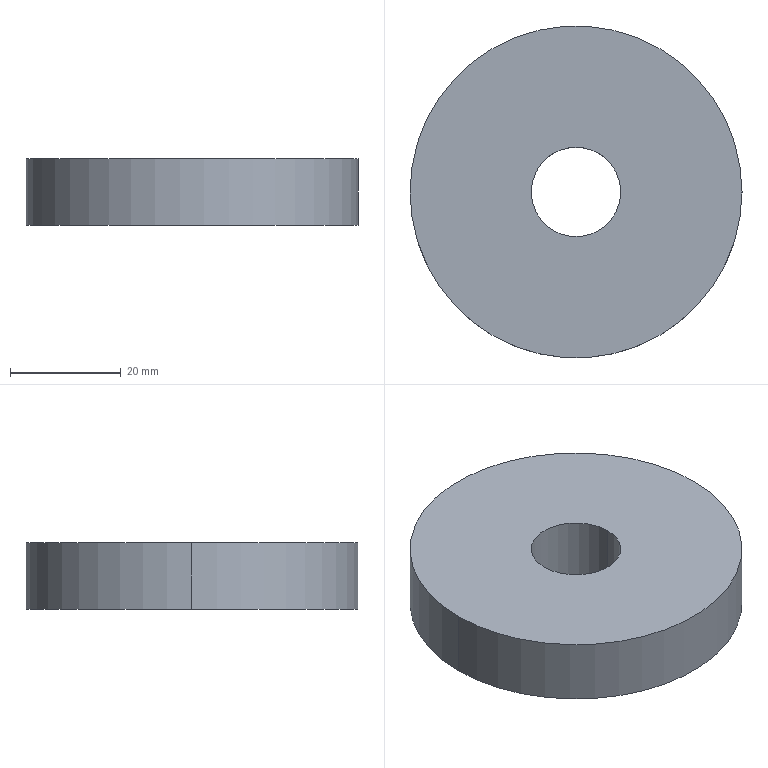Part | SolidWorks | features Extrusion 1 | 1 solid | 6 faces | box 60 x 60 x 12 mm | volume 31456 mm3 | cylinder 4 | plane 2 | commonest cylinder face diameters 16.2 x2 60 x2
STEP:
#1=CARTESIAN_POINT('',(-8.1,0.,-6.));
#2=VERTEX_POINT('',#1);
#3=CARTESIAN_POINT('',(8.1,0.,-6.));
#4=VERTEX_POINT('',#3);
#5=CARTESIAN_POINT('',(0.,0.,-6.));
#6=DIRECTION('',(0.,0.,1.));
#7=DIRECTION('',(1.,0.,0.));
#8=AXIS2_PLACEMENT_3D('',#5,#6,#7);
#9=CIRCLE('',#8,8.1);
#10=EDGE_CURVE('',#2,#4,#9,.T.);
#11=ORIENTED_EDGE('',*,*,#10,.F.);
#12=CARTESIAN_POINT('',(-8.1,0.,6.));
#13=VERTEX_POINT('',#12);
#14=CARTESIAN_POINT('',(-8.1,0.,-6.));
#15=DIRECTION('',(0.,0.,1.));
#16=VECTOR('',#15,1000.);
#17=LINE('',#14,#16);
#18=EDGE_CURVE('',#2,#13,#17,.T.);
#19=ORIENTED_EDGE('',*,*,#18,.T.);
#20=CARTESIAN_POINT('',(8.1,0.,6.));
#21=VERTEX_POINT('',#20);
#22=CARTESIAN_POINT('',(0.,0.,6.));
#23=DIRECTION('',(0.,0.,1.));
#24=DIRECTION('',(1.,0.,0.));
#25=AXIS2_PLACEMENT_3D('',#22,#23,#24);
#26=CIRCLE('',#25,8.1);
#27=EDGE_CURVE('',#13,#21,#26,.T.);
#28=ORIENTED_EDGE('',*,*,#27,.T.);
#29=CARTESIAN_POINT('',(8.1,0.,-6.));
#30=DIRECTION('',(0.,0.,1.));
#31=VECTOR('',#30,1000.);
#32=LINE('',#29,#31);
#33=EDGE_CURVE('',#4,#21,#32,.T.);
#34=ORIENTED_EDGE('',*,*,#33,.F.);
#35=EDGE_LOOP('',(#11,#19,#28,#34));
#36=FACE_OUTER_BOUND('',#35,.T.);
#37=CARTESIAN_POINT('',(0.,0.,-6.));
#38=DIRECTION('',(0.,0.,1.));
#39=DIRECTION('',(1.,0.,0.));
#40=AXIS2_PLACEMENT_3D('',#37,#38,#39);
#41=CYLINDRICAL_SURFACE('',#40,8.1);
#42=ADVANCED_FACE('',(#36),#41,.F.);
#43=CARTESIAN_POINT('',(30.,0.,-6.));
#44=VERTEX_POINT('',#43);
#45=CARTESIAN_POINT('',(-30.,0.,-6.));
#46=VERTEX_POINT('',#45);
#47=CARTESIAN_POINT('',(0.,0.,-6.));
#48=DIRECTION('',(0.,0.,1.));
#49=DIRECTION('',(1.,0.,0.));
#50=AXIS2_PLACEMENT_3D('',#47,#48,#49);
#51=CIRCLE('',#50,30.);
#52=EDGE_CURVE('',#44,#46,#51,.T.);
#53=ORIENTED_EDGE('',*,*,#52,.T.);
#54=CARTESIAN_POINT('',(-30.,0.,6.));
#55=VERTEX_POINT('',#54);
#56=CARTESIAN_POINT('',(-30.,0.,-6.));
#57=DIRECTION('',(0.,0.,1.));
#58=VECTOR('',#57,1000.);
#59=LINE('',#56,#58);
#60=EDGE_CURVE('',#46,#55,#59,.T.);
#61=ORIENTED_EDGE('',*,*,#60,.T.);
#62=CARTESIAN_POINT('',(30.,0.,6.));
#63=VERTEX_POINT('',#62);
#64=CARTESIAN_POINT('',(0.,0.,6.));
#65=DIRECTION('',(0.,0.,1.));
#66=DIRECTION('',(1.,0.,0.));
#67=AXIS2_PLACEMENT_3D('',#64,#65,#66);
#68=CIRCLE('',#67,30.);
#69=EDGE_CURVE('',#63,#55,#68,.T.);
#70=ORIENTED_EDGE('',*,*,#69,.F.);
#71=CARTESIAN_POINT('',(30.,0.,-6.));
#72=DIRECTION('',(0.,0.,1.));
#73=VECTOR('',#72,1000.);
#74=LINE('',#71,#73);
#75=EDGE_CURVE('',#44,#63,#74,.T.);
#76=ORIENTED_EDGE('',*,*,#75,.F.);
#77=EDGE_LOOP('',(#53,#61,#70,#76));
#78=FACE_OUTER_BOUND('',#77,.T.);
#79=CARTESIAN_POINT('',(0.,0.,-6.));
#80=DIRECTION('',(0.,0.,1.));
#81=DIRECTION('',(1.,0.,0.));
#82=AXIS2_PLACEMENT_3D('',#79,#80,#81);
#83=CYLINDRICAL_SURFACE('',#82,30.);
#84=ADVANCED_FACE('',(#78),#83,.T.);
#85=ORIENTED_EDGE('',*,*,#60,.F.);
#86=CARTESIAN_POINT('',(0.,0.,-6.));
#87=DIRECTION('',(0.,0.,1.));
#88=DIRECTION('',(1.,0.,0.));
#89=AXIS2_PLACEMENT_3D('',#86,#87,#88);
#90=CIRCLE('',#89,30.);
#91=EDGE_CURVE('',#46,#44,#90,.T.);
#92=ORIENTED_EDGE('',*,*,#91,.T.);
#93=ORIENTED_EDGE('',*,*,#75,.T.);
#94=CARTESIAN_POINT('',(0.,0.,6.));
#95=DIRECTION('',(0.,0.,1.));
#96=DIRECTION('',(1.,0.,0.));
#97=AXIS2_PLACEMENT_3D('',#94,#95,#96);
#98=CIRCLE('',#97,30.);
#99=EDGE_CURVE('',#55,#63,#98,.T.);
#100=ORIENTED_EDGE('',*,*,#99,.F.);
#101=EDGE_LOOP('',(#85,#92,#93,#100));
#102=FACE_OUTER_BOUND('',#101,.T.);
#103=CARTESIAN_POINT('',(0.,0.,-6.));
#104=DIRECTION('',(0.,0.,1.));
#105=DIRECTION('',(1.,0.,0.));
#106=AXIS2_PLACEMENT_3D('',#103,#104,#105);
#107=CYLINDRICAL_SURFACE('',#106,30.);
#108=ADVANCED_FACE('',(#102),#107,.T.);
#109=CARTESIAN_POINT('',(0.,0.,-6.));
#110=DIRECTION('',(0.,0.,1.));
#111=DIRECTION('',(1.,0.,0.));
#112=AXIS2_PLACEMENT_3D('',#109,#110,#111);
#113=CIRCLE('',#112,8.1);
#114=EDGE_CURVE('',#4,#2,#113,.T.);
#115=ORIENTED_EDGE('',*,*,#114,.T.);
#116=ORIENTED_EDGE('',*,*,#10,.T.);
#117=EDGE_LOOP('',(#115,#116));
#118=FACE_BOUND('',#117,.T.);
#119=ORIENTED_EDGE('',*,*,#52,.F.);
#120=ORIENTED_EDGE('',*,*,#91,.F.);
#121=EDGE_LOOP('',(#119,#120));
#122=FACE_OUTER_BOUND('',#121,.T.);
#123=CARTESIAN_POINT('',(0.,0.,-6.));
#124=DIRECTION('',(0.,0.,1.));
#125=DIRECTION('',(1.,0.,0.));
#126=AXIS2_PLACEMENT_3D('',#123,#124,#125);
#127=PLANE('',#126);
#128=ADVANCED_FACE('',(#118,#122),#127,.F.);
#129=CARTESIAN_POINT('',(0.,0.,6.));
#130=DIRECTION('',(0.,0.,1.));
#131=DIRECTION('',(1.,0.,0.));
#132=AXIS2_PLACEMENT_3D('',#129,#130,#131);
#133=CIRCLE('',#132,8.1);
#134=EDGE_CURVE('',#21,#13,#133,.T.);
#135=ORIENTED_EDGE('',*,*,#134,.F.);
#136=ORIENTED_EDGE('',*,*,#27,.F.);
#137=EDGE_LOOP('',(#135,#136));
#138=FACE_BOUND('',#137,.T.);
#139=ORIENTED_EDGE('',*,*,#69,.T.);
#140=ORIENTED_EDGE('',*,*,#99,.T.);
#141=EDGE_LOOP('',(#139,#140));
#142=FACE_OUTER_BOUND('',#141,.T.);
#143=CARTESIAN_POINT('',(0.,0.,6.));
#144=DIRECTION('',(0.,0.,1.));
#145=DIRECTION('',(1.,0.,0.));
#146=AXIS2_PLACEMENT_3D('',#143,#144,#145);
#147=PLANE('',#146);
#148=ADVANCED_FACE('',(#138,#142),#147,.T.);
#149=ORIENTED_EDGE('',*,*,#18,.F.);
#150=ORIENTED_EDGE('',*,*,#114,.F.);
#151=ORIENTED_EDGE('',*,*,#33,.T.);
#152=ORIENTED_EDGE('',*,*,#134,.T.);
#153=EDGE_LOOP('',(#149,#150,#151,#152));
#154=FACE_OUTER_BOUND('',#153,.T.);
#155=CARTESIAN_POINT('',(0.,0.,-6.));
#156=DIRECTION('',(0.,0.,1.));
#157=DIRECTION('',(1.,0.,0.));
#158=AXIS2_PLACEMENT_3D('',#155,#156,#157);
#159=CYLINDRICAL_SURFACE('',#158,8.1);
#160=ADVANCED_FACE('',(#154),#159,.F.);
#161=CLOSED_SHELL('',(#42,#84,#108,#128,#148,#160));
#162=MANIFOLD_SOLID_BREP('',#161);
#163=CARTESIAN_POINT('',(0.,0.,0.));
#164=DIRECTION('',(0.,0.,1.));
#165=DIRECTION('',(1.,0.,0.));
#166=AXIS2_PLACEMENT_3D('',#163,#164,#165);
#167=(LENGTH_UNIT()NAMED_UNIT(*)SI_UNIT(.MILLI.,.METRE.));
#168=UNCERTAINTY_MEASURE_WITH_UNIT(LENGTH_MEASURE(0.00001),#167,'','');
#169=(NAMED_UNIT(*)PLANE_ANGLE_UNIT()SI_UNIT($,.RADIAN.));
#170=(NAMED_UNIT(*)SI_UNIT($,.STERADIAN.)SOLID_ANGLE_UNIT());
#171=(GEOMETRIC_REPRESENTATION_CONTEXT(3)GLOBAL_UNCERTAINTY_ASSIGNED_CONTEXT((#168))GLOBAL_UNIT_ASSIGNED_CONTEXT((#167,#169,#170))REPRESENTATION_CONTEXT('',''));
#172=ADVANCED_BREP_SHAPE_REPRESENTATION('',(#162,#166),#171);